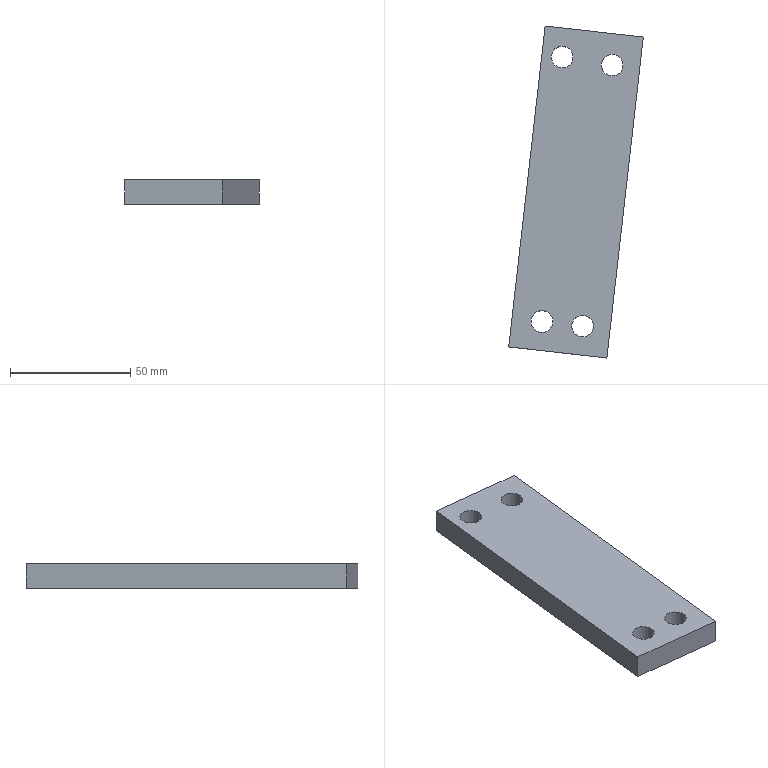Part | NX | features solid 2 | 1 solid | 10 faces | box 55.812 x 137.761 x 10 mm | volume 52395 mm3 | plane 6 | cylinder 4 | commonest cylinder face diameters 9 x4
STEP:
#1=CARTESIAN_POINT('',(237.879,-333.435,30.));
#2=VERTEX_POINT('',#1);
#3=CARTESIAN_POINT('',(252.951,-200.285,30.));
#4=VERTEX_POINT('',#3);
#5=CARTESIAN_POINT('',(214.764,-537.629,30.));
#6=DIRECTION('',(0.1125,0.9937,0.));
#7=VECTOR('',#6,1000.);
#8=LINE('',#5,#7);
#9=EDGE_CURVE('',#2,#4,#8,.T.);
#10=ORIENTED_EDGE('',*,*,#9,.T.);
#11=CARTESIAN_POINT('',(252.951,-200.285,40.));
#12=VERTEX_POINT('',#11);
#13=CARTESIAN_POINT('',(252.951,-200.285,40.));
#14=DIRECTION('',(0.,0.,-1.));
#15=VECTOR('',#14,1000.);
#16=LINE('',#13,#15);
#17=EDGE_CURVE('',#12,#4,#16,.T.);
#18=ORIENTED_EDGE('',*,*,#17,.F.);
#19=CARTESIAN_POINT('',(237.879,-333.435,40.));
#20=VERTEX_POINT('',#19);
#21=CARTESIAN_POINT('',(214.764,-537.629,40.));
#22=DIRECTION('',(0.1125,0.9937,0.));
#23=VECTOR('',#22,1000.);
#24=LINE('',#21,#23);
#25=EDGE_CURVE('',#20,#12,#24,.T.);
#26=ORIENTED_EDGE('',*,*,#25,.F.);
#27=CARTESIAN_POINT('',(237.879,-333.435,40.));
#28=DIRECTION('',(0.,0.,-1.));
#29=VECTOR('',#28,1000.);
#30=LINE('',#27,#29);
#31=EDGE_CURVE('',#20,#2,#30,.T.);
#32=ORIENTED_EDGE('',*,*,#31,.T.);
#33=EDGE_LOOP('',(#10,#18,#26,#32));
#34=FACE_BOUND('',#33,.T.);
#35=CARTESIAN_POINT('',(214.764,-537.629,40.));
#36=DIRECTION('',(-0.9937,0.1125,0.));
#37=DIRECTION('',(0.1125,0.9937,0.));
#38=AXIS2_PLACEMENT_3D('',#35,#36,#37);
#39=PLANE('',#38);
#40=ADVANCED_FACE('',(#34),#39,.F.);
#41=CARTESIAN_POINT('',(212.211,-195.673,30.));
#42=VERTEX_POINT('',#41);
#43=CARTESIAN_POINT('',(458.458,-223.548,30.));
#44=DIRECTION('',(-0.9937,0.1125,0.));
#45=VECTOR('',#44,1000.);
#46=LINE('',#43,#45);
#47=EDGE_CURVE('',#4,#42,#46,.T.);
#48=ORIENTED_EDGE('',*,*,#47,.T.);
#49=CARTESIAN_POINT('',(212.211,-195.673,40.));
#50=VERTEX_POINT('',#49);
#51=CARTESIAN_POINT('',(212.211,-195.673,40.));
#52=DIRECTION('',(0.,0.,-1.));
#53=VECTOR('',#52,1000.);
#54=LINE('',#51,#53);
#55=EDGE_CURVE('',#50,#42,#54,.T.);
#56=ORIENTED_EDGE('',*,*,#55,.F.);
#57=CARTESIAN_POINT('',(458.458,-223.548,40.));
#58=DIRECTION('',(-0.9937,0.1125,0.));
#59=VECTOR('',#58,1000.);
#60=LINE('',#57,#59);
#61=EDGE_CURVE('',#12,#50,#60,.T.);
#62=ORIENTED_EDGE('',*,*,#61,.F.);
#63=ORIENTED_EDGE('',*,*,#17,.T.);
#64=EDGE_LOOP('',(#48,#56,#62,#63));
#65=FACE_BOUND('',#64,.T.);
#66=CARTESIAN_POINT('',(458.458,-223.548,40.));
#67=DIRECTION('',(-0.1125,-0.9937,0.));
#68=DIRECTION('',(-0.9937,0.1125,0.));
#69=AXIS2_PLACEMENT_3D('',#66,#67,#68);
#70=PLANE('',#69);
#71=ADVANCED_FACE('',(#65),#70,.F.);
#72=CARTESIAN_POINT('',(197.139,-328.823,30.));
#73=VERTEX_POINT('',#72);
#74=CARTESIAN_POINT('',(174.024,-533.017,30.));
#75=DIRECTION('',(-0.1125,-0.9937,0.));
#76=VECTOR('',#75,1000.);
#77=LINE('',#74,#76);
#78=EDGE_CURVE('',#42,#73,#77,.T.);
#79=ORIENTED_EDGE('',*,*,#78,.T.);
#80=CARTESIAN_POINT('',(197.139,-328.823,40.));
#81=VERTEX_POINT('',#80);
#82=CARTESIAN_POINT('',(197.139,-328.823,40.));
#83=DIRECTION('',(0.,0.,-1.));
#84=VECTOR('',#83,1000.);
#85=LINE('',#82,#84);
#86=EDGE_CURVE('',#81,#73,#85,.T.);
#87=ORIENTED_EDGE('',*,*,#86,.F.);
#88=CARTESIAN_POINT('',(174.024,-533.017,40.));
#89=DIRECTION('',(-0.1125,-0.9937,0.));
#90=VECTOR('',#89,1000.);
#91=LINE('',#88,#90);
#92=EDGE_CURVE('',#50,#81,#91,.T.);
#93=ORIENTED_EDGE('',*,*,#92,.F.);
#94=ORIENTED_EDGE('',*,*,#55,.T.);
#95=EDGE_LOOP('',(#79,#87,#93,#94));
#96=FACE_BOUND('',#95,.T.);
#97=CARTESIAN_POINT('',(174.024,-533.017,40.));
#98=DIRECTION('',(0.9937,-0.1125,0.));
#99=DIRECTION('',(-0.1125,-0.9937,0.));
#100=AXIS2_PLACEMENT_3D('',#97,#98,#99);
#101=PLANE('',#100);
#102=ADVANCED_FACE('',(#96),#101,.F.);
#103=CARTESIAN_POINT('',(227.801,-315.717,40.));
#104=VERTEX_POINT('',#103);
#105=CARTESIAN_POINT('',(227.801,-320.217,40.));
#106=DIRECTION('',(0.,0.,-1.));
#107=DIRECTION('',(0.,1.,0.));
#108=AXIS2_PLACEMENT_3D('',#105,#106,#107);
#109=CIRCLE('',#108,4.5);
#110=EDGE_CURVE('',#104,#104,#109,.T.);
#111=ORIENTED_EDGE('',*,*,#110,.F.);
#112=EDGE_LOOP('',(#111));
#113=FACE_BOUND('',#112,.T.);
#114=CARTESIAN_POINT('',(227.801,-315.717,30.));
#115=VERTEX_POINT('',#114);
#116=CARTESIAN_POINT('',(227.801,-320.217,30.));
#117=DIRECTION('',(0.,0.,-1.));
#118=DIRECTION('',(0.,1.,0.));
#119=AXIS2_PLACEMENT_3D('',#116,#117,#118);
#120=CIRCLE('',#119,4.5);
#121=EDGE_CURVE('',#115,#115,#120,.T.);
#122=ORIENTED_EDGE('',*,*,#121,.T.);
#123=EDGE_LOOP('',(#122));
#124=FACE_BOUND('',#123,.T.);
#125=CARTESIAN_POINT('',(227.801,-320.217,40.));
#126=DIRECTION('',(0.,0.,-1.));
#127=DIRECTION('',(0.,-1.,0.));
#128=AXIS2_PLACEMENT_3D('',#125,#126,#127);
#129=CYLINDRICAL_SURFACE('',#128,4.5);
#130=ADVANCED_FACE('',(#113,#124),#129,.F.);
#131=CARTESIAN_POINT('',(210.909,-313.805,40.));
#132=VERTEX_POINT('',#131);
#133=CARTESIAN_POINT('',(210.909,-318.305,40.));
#134=DIRECTION('',(0.,0.,-1.));
#135=DIRECTION('',(0.,1.,0.));
#136=AXIS2_PLACEMENT_3D('',#133,#134,#135);
#137=CIRCLE('',#136,4.5);
#138=EDGE_CURVE('',#132,#132,#137,.T.);
#139=ORIENTED_EDGE('',*,*,#138,.F.);
#140=EDGE_LOOP('',(#139));
#141=FACE_BOUND('',#140,.T.);
#142=CARTESIAN_POINT('',(210.909,-313.805,30.));
#143=VERTEX_POINT('',#142);
#144=CARTESIAN_POINT('',(210.909,-318.305,30.));
#145=DIRECTION('',(0.,0.,-1.));
#146=DIRECTION('',(0.,1.,0.));
#147=AXIS2_PLACEMENT_3D('',#144,#145,#146);
#148=CIRCLE('',#147,4.5);
#149=EDGE_CURVE('',#143,#143,#148,.T.);
#150=ORIENTED_EDGE('',*,*,#149,.T.);
#151=EDGE_LOOP('',(#150));
#152=FACE_BOUND('',#151,.T.);
#153=CARTESIAN_POINT('',(210.909,-318.305,40.));
#154=DIRECTION('',(0.,0.,-1.));
#155=DIRECTION('',(0.,-1.,0.));
#156=AXIS2_PLACEMENT_3D('',#153,#154,#155);
#157=CYLINDRICAL_SURFACE('',#156,4.5);
#158=ADVANCED_FACE('',(#141,#152),#157,.F.);
#159=CARTESIAN_POINT('',(240.062,-207.409,40.));
#160=VERTEX_POINT('',#159);
#161=CARTESIAN_POINT('',(240.062,-211.909,40.));
#162=DIRECTION('',(0.,0.,1.));
#163=DIRECTION('',(0.,1.,0.));
#164=AXIS2_PLACEMENT_3D('',#161,#162,#163);
#165=CIRCLE('',#164,4.5);
#166=EDGE_CURVE('',#160,#160,#165,.T.);
#167=ORIENTED_EDGE('',*,*,#166,.T.);
#168=EDGE_LOOP('',(#167));
#169=FACE_BOUND('',#168,.T.);
#170=CARTESIAN_POINT('',(240.062,-207.409,30.));
#171=VERTEX_POINT('',#170);
#172=CARTESIAN_POINT('',(240.062,-211.909,30.));
#173=DIRECTION('',(0.,0.,1.));
#174=DIRECTION('',(0.,1.,0.));
#175=AXIS2_PLACEMENT_3D('',#172,#173,#174);
#176=CIRCLE('',#175,4.5);
#177=EDGE_CURVE('',#171,#171,#176,.T.);
#178=ORIENTED_EDGE('',*,*,#177,.F.);
#179=EDGE_LOOP('',(#178));
#180=FACE_BOUND('',#179,.T.);
#181=CARTESIAN_POINT('',(240.062,-211.909,40.));
#182=DIRECTION('',(0.,0.,-1.));
#183=DIRECTION('',(0.,-1.,0.));
#184=AXIS2_PLACEMENT_3D('',#181,#182,#183);
#185=CYLINDRICAL_SURFACE('',#184,4.5);
#186=ADVANCED_FACE('',(#169,#180),#185,.F.);
#187=CARTESIAN_POINT('',(443.385,-356.698,30.));
#188=DIRECTION('',(0.9937,-0.1125,0.));
#189=VECTOR('',#188,1000.);
#190=LINE('',#187,#189);
#191=EDGE_CURVE('',#73,#2,#190,.T.);
#192=ORIENTED_EDGE('',*,*,#191,.T.);
#193=ORIENTED_EDGE('',*,*,#31,.F.);
#194=CARTESIAN_POINT('',(443.385,-356.698,40.));
#195=DIRECTION('',(0.9937,-0.1125,0.));
#196=VECTOR('',#195,1000.);
#197=LINE('',#194,#196);
#198=EDGE_CURVE('',#81,#20,#197,.T.);
#199=ORIENTED_EDGE('',*,*,#198,.F.);
#200=ORIENTED_EDGE('',*,*,#86,.T.);
#201=EDGE_LOOP('',(#192,#193,#199,#200));
#202=FACE_BOUND('',#201,.T.);
#203=CARTESIAN_POINT('',(443.385,-356.698,40.));
#204=DIRECTION('',(0.1125,0.9937,0.));
#205=DIRECTION('',(0.9937,-0.1125,0.));
#206=AXIS2_PLACEMENT_3D('',#203,#204,#205);
#207=PLANE('',#206);
#208=ADVANCED_FACE('',(#202),#207,.F.);
#209=CARTESIAN_POINT('',(219.308,-204.053,40.));
#210=VERTEX_POINT('',#209);
#211=CARTESIAN_POINT('',(219.308,-208.553,40.));
#212=DIRECTION('',(0.,0.,1.));
#213=DIRECTION('',(0.,1.,0.));
#214=AXIS2_PLACEMENT_3D('',#211,#212,#213);
#215=CIRCLE('',#214,4.5);
#216=EDGE_CURVE('',#210,#210,#215,.T.);
#217=ORIENTED_EDGE('',*,*,#216,.T.);
#218=EDGE_LOOP('',(#217));
#219=FACE_BOUND('',#218,.T.);
#220=CARTESIAN_POINT('',(219.308,-204.053,30.));
#221=VERTEX_POINT('',#220);
#222=CARTESIAN_POINT('',(219.308,-208.553,30.));
#223=DIRECTION('',(0.,0.,1.));
#224=DIRECTION('',(0.,1.,0.));
#225=AXIS2_PLACEMENT_3D('',#222,#223,#224);
#226=CIRCLE('',#225,4.5);
#227=EDGE_CURVE('',#221,#221,#226,.T.);
#228=ORIENTED_EDGE('',*,*,#227,.F.);
#229=EDGE_LOOP('',(#228));
#230=FACE_BOUND('',#229,.T.);
#231=CARTESIAN_POINT('',(219.308,-208.553,40.));
#232=DIRECTION('',(0.,0.,-1.));
#233=DIRECTION('',(0.,-1.,0.));
#234=AXIS2_PLACEMENT_3D('',#231,#232,#233);
#235=CYLINDRICAL_SURFACE('',#234,4.5);
#236=ADVANCED_FACE('',(#219,#230),#235,.F.);
#237=ORIENTED_EDGE('',*,*,#25,.T.);
#238=ORIENTED_EDGE('',*,*,#61,.T.);
#239=ORIENTED_EDGE('',*,*,#92,.T.);
#240=ORIENTED_EDGE('',*,*,#198,.T.);
#241=EDGE_LOOP('',(#237,#238,#239,#240));
#242=FACE_BOUND('',#241,.T.);
#243=ORIENTED_EDGE('',*,*,#166,.F.);
#244=EDGE_LOOP('',(#243));
#245=FACE_BOUND('',#244,.T.);
#246=ORIENTED_EDGE('',*,*,#138,.T.);
#247=EDGE_LOOP('',(#246));
#248=FACE_BOUND('',#247,.T.);
#249=ORIENTED_EDGE('',*,*,#110,.T.);
#250=EDGE_LOOP('',(#249));
#251=FACE_BOUND('',#250,.T.);
#252=ORIENTED_EDGE('',*,*,#216,.F.);
#253=EDGE_LOOP('',(#252));
#254=FACE_BOUND('',#253,.T.);
#255=CARTESIAN_POINT('',(427.226,-561.68,40.));
#256=DIRECTION('',(0.,0.,-1.));
#257=DIRECTION('',(-0.9981,-0.06177,0.));
#258=AXIS2_PLACEMENT_3D('',#255,#256,#257);
#259=PLANE('',#258);
#260=ADVANCED_FACE('',(#242,#245,#248,#251,#254),#259,.F.);
#261=ORIENTED_EDGE('',*,*,#9,.F.);
#262=ORIENTED_EDGE('',*,*,#191,.F.);
#263=ORIENTED_EDGE('',*,*,#78,.F.);
#264=ORIENTED_EDGE('',*,*,#47,.F.);
#265=EDGE_LOOP('',(#261,#262,#263,#264));
#266=FACE_BOUND('',#265,.T.);
#267=ORIENTED_EDGE('',*,*,#177,.T.);
#268=EDGE_LOOP('',(#267));
#269=FACE_BOUND('',#268,.T.);
#270=ORIENTED_EDGE('',*,*,#149,.F.);
#271=EDGE_LOOP('',(#270));
#272=FACE_BOUND('',#271,.T.);
#273=ORIENTED_EDGE('',*,*,#121,.F.);
#274=EDGE_LOOP('',(#273));
#275=FACE_BOUND('',#274,.T.);
#276=ORIENTED_EDGE('',*,*,#227,.T.);
#277=EDGE_LOOP('',(#276));
#278=FACE_BOUND('',#277,.T.);
#279=CARTESIAN_POINT('',(427.226,-561.68,30.));
#280=DIRECTION('',(0.,0.,-1.));
#281=DIRECTION('',(-0.9981,-0.06177,0.));
#282=AXIS2_PLACEMENT_3D('',#279,#280,#281);
#283=PLANE('',#282);
#284=ADVANCED_FACE('',(#266,#269,#272,#275,#278),#283,.T.);
#285=CLOSED_SHELL('',(#40,#71,#102,#130,#158,#186,#208,#236,#260,#284));
#286=MANIFOLD_SOLID_BREP('',#285);
#287=(LENGTH_UNIT()NAMED_UNIT(*)SI_UNIT(.MILLI.,.METRE.));
#288=UNCERTAINTY_MEASURE_WITH_UNIT(LENGTH_MEASURE(0.00001),#287,'','');
#289=(NAMED_UNIT(*)PLANE_ANGLE_UNIT()SI_UNIT($,.RADIAN.));
#290=(NAMED_UNIT(*)SI_UNIT($,.STERADIAN.)SOLID_ANGLE_UNIT());
#291=(GEOMETRIC_REPRESENTATION_CONTEXT(3)GLOBAL_UNCERTAINTY_ASSIGNED_CONTEXT((#288))GLOBAL_UNIT_ASSIGNED_CONTEXT((#287,#289,#290))REPRESENTATION_CONTEXT('',''));
#292=ADVANCED_BREP_SHAPE_REPRESENTATION('',(#286),#291);